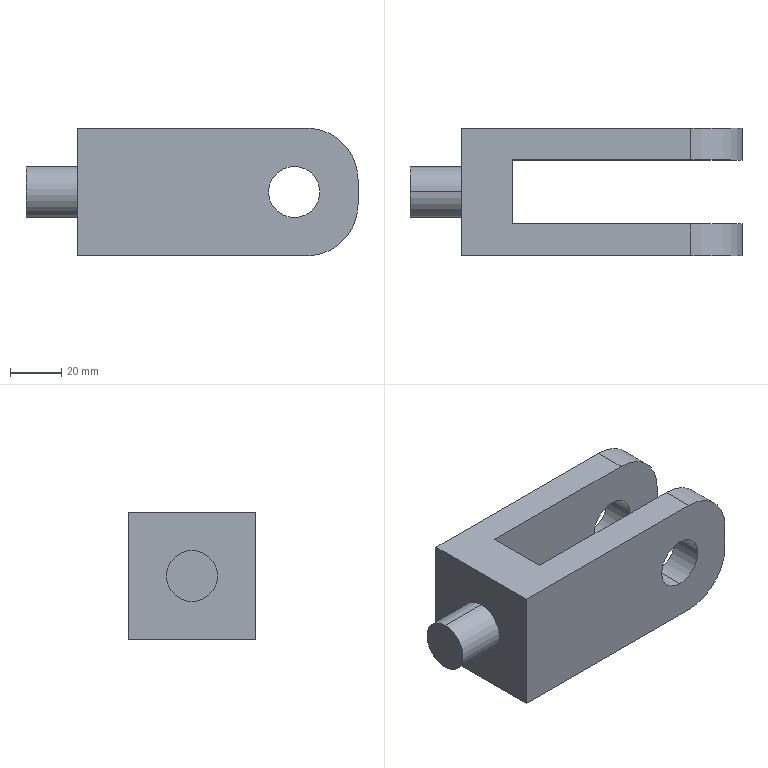Part | SolidWorks | 1 solid | 21 faces | box 130 x 50 x 50 mm | volume 156637 mm3 | plane 11 | cylinder 10 | commonest cylinder face diameters 20 x6 40 x4
STEP:
#1=CARTESIAN_POINT('',(-75.,25.,10.));
#2=VERTEX_POINT('',#1);
#3=CARTESIAN_POINT('',(-75.,25.,-10.));
#4=VERTEX_POINT('',#3);
#5=CARTESIAN_POINT('',(-75.,25.,0.));
#6=DIRECTION('',(-1.,0.,0.));
#7=DIRECTION('',(0.,0.,1.));
#8=AXIS2_PLACEMENT_3D('',#5,#6,#7);
#9=CIRCLE('',#8,10.);
#10=EDGE_CURVE('',#2,#4,#9,.T.);
#11=ORIENTED_EDGE('',*,*,#10,.F.);
#12=CARTESIAN_POINT('',(-55.,25.,10.));
#13=VERTEX_POINT('',#12);
#14=CARTESIAN_POINT('',(-75.,25.,10.));
#15=DIRECTION('',(1.,0.,0.));
#16=VECTOR('',#15,1000.);
#17=LINE('',#14,#16);
#18=EDGE_CURVE('',#2,#13,#17,.T.);
#19=ORIENTED_EDGE('',*,*,#18,.T.);
#20=CARTESIAN_POINT('',(-55.,25.,-10.));
#21=VERTEX_POINT('',#20);
#22=CARTESIAN_POINT('',(-55.,25.,0.));
#23=DIRECTION('',(-1.,0.,0.));
#24=DIRECTION('',(0.,0.,1.));
#25=AXIS2_PLACEMENT_3D('',#22,#23,#24);
#26=CIRCLE('',#25,10.);
#27=EDGE_CURVE('',#13,#21,#26,.T.);
#28=ORIENTED_EDGE('',*,*,#27,.T.);
#29=CARTESIAN_POINT('',(-75.,25.,-10.));
#30=DIRECTION('',(1.,0.,0.));
#31=VECTOR('',#30,1000.);
#32=LINE('',#29,#31);
#33=EDGE_CURVE('',#4,#21,#32,.T.);
#34=ORIENTED_EDGE('',*,*,#33,.F.);
#35=EDGE_LOOP('',(#11,#19,#28,#34));
#36=FACE_OUTER_BOUND('',#35,.T.);
#37=CARTESIAN_POINT('',(-75.,25.,0.));
#38=DIRECTION('',(1.,0.,0.));
#39=DIRECTION('',(0.,0.,-1.));
#40=AXIS2_PLACEMENT_3D('',#37,#38,#39);
#41=CYLINDRICAL_SURFACE('',#40,10.);
#42=ADVANCED_FACE('',(#36),#41,.T.);
#43=CARTESIAN_POINT('',(30.,12.5,10.));
#44=VERTEX_POINT('',#43);
#45=CARTESIAN_POINT('',(30.,12.5,-10.));
#46=VERTEX_POINT('',#45);
#47=CARTESIAN_POINT('',(30.,12.5,0.));
#48=DIRECTION('',(0.,-1.,0.));
#49=DIRECTION('',(0.,0.,-1.));
#50=AXIS2_PLACEMENT_3D('',#47,#48,#49);
#51=CIRCLE('',#50,10.);
#52=EDGE_CURVE('',#44,#46,#51,.T.);
#53=ORIENTED_EDGE('',*,*,#52,.F.);
#54=CARTESIAN_POINT('',(30.,0.,10.));
#55=VERTEX_POINT('',#54);
#56=CARTESIAN_POINT('',(30.,90.,10.));
#57=DIRECTION('',(0.,-1.,0.));
#58=VECTOR('',#57,1000.);
#59=LINE('',#56,#58);
#60=EDGE_CURVE('',#44,#55,#59,.T.);
#61=ORIENTED_EDGE('',*,*,#60,.T.);
#62=CARTESIAN_POINT('',(30.,0.,-10.));
#63=VERTEX_POINT('',#62);
#64=CARTESIAN_POINT('',(30.,0.,0.));
#65=DIRECTION('',(0.,-1.,0.));
#66=DIRECTION('',(0.,0.,-1.));
#67=AXIS2_PLACEMENT_3D('',#64,#65,#66);
#68=CIRCLE('',#67,10.);
#69=EDGE_CURVE('',#55,#63,#68,.T.);
#70=ORIENTED_EDGE('',*,*,#69,.T.);
#71=CARTESIAN_POINT('',(30.,90.,-10.));
#72=DIRECTION('',(0.,-1.,0.));
#73=VECTOR('',#72,1000.);
#74=LINE('',#71,#73);
#75=EDGE_CURVE('',#46,#63,#74,.T.);
#76=ORIENTED_EDGE('',*,*,#75,.F.);
#77=EDGE_LOOP('',(#53,#61,#70,#76));
#78=FACE_OUTER_BOUND('',#77,.T.);
#79=CARTESIAN_POINT('',(30.,90.,0.));
#80=DIRECTION('',(0.,-1.,0.));
#81=DIRECTION('',(0.,0.,-1.));
#82=AXIS2_PLACEMENT_3D('',#79,#80,#81);
#83=CYLINDRICAL_SURFACE('',#82,10.);
#84=ADVANCED_FACE('',(#78),#83,.F.);
#85=CARTESIAN_POINT('',(30.,50.,-10.));
#86=VERTEX_POINT('',#85);
#87=CARTESIAN_POINT('',(30.,50.,10.));
#88=VERTEX_POINT('',#87);
#89=CARTESIAN_POINT('',(30.,50.,0.));
#90=DIRECTION('',(0.,1.,0.));
#91=DIRECTION('',(0.,0.,1.));
#92=AXIS2_PLACEMENT_3D('',#89,#90,#91);
#93=CIRCLE('',#92,10.);
#94=EDGE_CURVE('',#86,#88,#93,.T.);
#95=ORIENTED_EDGE('',*,*,#94,.T.);
#96=CARTESIAN_POINT('',(30.,37.5,10.));
#97=VERTEX_POINT('',#96);
#98=CARTESIAN_POINT('',(30.,90.,10.));
#99=DIRECTION('',(0.,-1.,0.));
#100=VECTOR('',#99,1000.);
#101=LINE('',#98,#100);
#102=EDGE_CURVE('',#88,#97,#101,.T.);
#103=ORIENTED_EDGE('',*,*,#102,.T.);
#104=CARTESIAN_POINT('',(30.,37.5,-10.));
#105=VERTEX_POINT('',#104);
#106=CARTESIAN_POINT('',(30.,37.5,0.));
#107=DIRECTION('',(0.,1.,0.));
#108=DIRECTION('',(0.,0.,1.));
#109=AXIS2_PLACEMENT_3D('',#106,#107,#108);
#110=CIRCLE('',#109,10.);
#111=EDGE_CURVE('',#105,#97,#110,.T.);
#112=ORIENTED_EDGE('',*,*,#111,.F.);
#113=CARTESIAN_POINT('',(30.,90.,-10.));
#114=DIRECTION('',(0.,-1.,0.));
#115=VECTOR('',#114,1000.);
#116=LINE('',#113,#115);
#117=EDGE_CURVE('',#86,#105,#116,.T.);
#118=ORIENTED_EDGE('',*,*,#117,.F.);
#119=EDGE_LOOP('',(#95,#103,#112,#118));
#120=FACE_OUTER_BOUND('',#119,.T.);
#121=CARTESIAN_POINT('',(30.,90.,0.));
#122=DIRECTION('',(0.,-1.,0.));
#123=DIRECTION('',(0.,0.,-1.));
#124=AXIS2_PLACEMENT_3D('',#121,#122,#123);
#125=CYLINDRICAL_SURFACE('',#124,10.);
#126=ADVANCED_FACE('',(#120),#125,.F.);
#127=CARTESIAN_POINT('',(55.,0.,5.));
#128=VERTEX_POINT('',#127);
#129=CARTESIAN_POINT('',(55.,0.,-5.));
#130=VERTEX_POINT('',#129);
#131=CARTESIAN_POINT('',(55.,0.,-25.));
#132=DIRECTION('',(0.,0.,-1.));
#133=VECTOR('',#132,1000.);
#134=LINE('',#131,#133);
#135=EDGE_CURVE('',#128,#130,#134,.T.);
#136=ORIENTED_EDGE('',*,*,#135,.T.);
#137=CARTESIAN_POINT('',(55.,12.5,-5.));
#138=VERTEX_POINT('',#137);
#139=CARTESIAN_POINT('',(55.,50.,-5.));
#140=DIRECTION('',(0.,1.,0.));
#141=VECTOR('',#140,1000.);
#142=LINE('',#139,#141);
#143=EDGE_CURVE('',#130,#138,#142,.T.);
#144=ORIENTED_EDGE('',*,*,#143,.T.);
#145=CARTESIAN_POINT('',(55.,12.5,5.));
#146=VERTEX_POINT('',#145);
#147=CARTESIAN_POINT('',(55.,12.5,25.));
#148=DIRECTION('',(0.,0.,-1.));
#149=VECTOR('',#148,1000.);
#150=LINE('',#147,#149);
#151=EDGE_CURVE('',#146,#138,#150,.T.);
#152=ORIENTED_EDGE('',*,*,#151,.F.);
#153=CARTESIAN_POINT('',(55.,50.,5.));
#154=DIRECTION('',(0.,-1.,0.));
#155=VECTOR('',#154,1000.);
#156=LINE('',#153,#155);
#157=EDGE_CURVE('',#146,#128,#156,.T.);
#158=ORIENTED_EDGE('',*,*,#157,.T.);
#159=EDGE_LOOP('',(#136,#144,#152,#158));
#160=FACE_OUTER_BOUND('',#159,.T.);
#161=CARTESIAN_POINT('',(55.,50.,-25.));
#162=DIRECTION('',(-1.,0.,0.));
#163=DIRECTION('',(0.,0.,1.));
#164=AXIS2_PLACEMENT_3D('',#161,#162,#163);
#165=PLANE('',#164);
#166=ADVANCED_FACE('',(#160),#165,.F.);
#167=CARTESIAN_POINT('',(55.,37.5,-5.));
#168=VERTEX_POINT('',#167);
#169=CARTESIAN_POINT('',(55.,37.5,5.));
#170=VERTEX_POINT('',#169);
#171=CARTESIAN_POINT('',(55.,37.5,25.));
#172=DIRECTION('',(0.,0.,1.));
#173=VECTOR('',#172,1000.);
#174=LINE('',#171,#173);
#175=EDGE_CURVE('',#168,#170,#174,.T.);
#176=ORIENTED_EDGE('',*,*,#175,.F.);
#177=CARTESIAN_POINT('',(55.,50.,-5.));
#178=VERTEX_POINT('',#177);
#179=CARTESIAN_POINT('',(55.,50.,-5.));
#180=DIRECTION('',(0.,1.,0.));
#181=VECTOR('',#180,1000.);
#182=LINE('',#179,#181);
#183=EDGE_CURVE('',#168,#178,#182,.T.);
#184=ORIENTED_EDGE('',*,*,#183,.T.);
#185=CARTESIAN_POINT('',(55.,50.,5.));
#186=VERTEX_POINT('',#185);
#187=CARTESIAN_POINT('',(55.,50.,-25.));
#188=DIRECTION('',(0.,0.,-1.));
#189=VECTOR('',#188,1000.);
#190=LINE('',#187,#189);
#191=EDGE_CURVE('',#186,#178,#190,.T.);
#192=ORIENTED_EDGE('',*,*,#191,.F.);
#193=CARTESIAN_POINT('',(55.,50.,5.));
#194=DIRECTION('',(0.,-1.,0.));
#195=VECTOR('',#194,1000.);
#196=LINE('',#193,#195);
#197=EDGE_CURVE('',#186,#170,#196,.T.);
#198=ORIENTED_EDGE('',*,*,#197,.T.);
#199=EDGE_LOOP('',(#176,#184,#192,#198));
#200=FACE_OUTER_BOUND('',#199,.T.);
#201=CARTESIAN_POINT('',(55.,50.,-25.));
#202=DIRECTION('',(-1.,0.,0.));
#203=DIRECTION('',(0.,0.,1.));
#204=AXIS2_PLACEMENT_3D('',#201,#202,#203);
#205=PLANE('',#204);
#206=ADVANCED_FACE('',(#200),#205,.F.);
#207=CARTESIAN_POINT('',(-35.,12.5,-25.));
#208=VERTEX_POINT('',#207);
#209=CARTESIAN_POINT('',(35.,12.5,-25.));
#210=VERTEX_POINT('',#209);
#211=CARTESIAN_POINT('',(-35.,12.5,-25.));
#212=DIRECTION('',(1.,0.,0.));
#213=VECTOR('',#212,1000.);
#214=LINE('',#211,#213);
#215=EDGE_CURVE('',#208,#210,#214,.T.);
#216=ORIENTED_EDGE('',*,*,#215,.T.);
#217=CARTESIAN_POINT('',(35.,0.,-25.));
#218=VERTEX_POINT('',#217);
#219=CARTESIAN_POINT('',(35.,50.,-25.));
#220=DIRECTION('',(0.,-1.,0.));
#221=VECTOR('',#220,1000.);
#222=LINE('',#219,#221);
#223=EDGE_CURVE('',#210,#218,#222,.T.);
#224=ORIENTED_EDGE('',*,*,#223,.T.);
#225=CARTESIAN_POINT('',(-55.,0.,-25.));
#226=VERTEX_POINT('',#225);
#227=CARTESIAN_POINT('',(-55.,0.,-25.));
#228=DIRECTION('',(-1.,0.,0.));
#229=VECTOR('',#228,1000.);
#230=LINE('',#227,#229);
#231=EDGE_CURVE('',#218,#226,#230,.T.);
#232=ORIENTED_EDGE('',*,*,#231,.T.);
#233=CARTESIAN_POINT('',(-55.,50.,-25.));
#234=VERTEX_POINT('',#233);
#235=CARTESIAN_POINT('',(-55.,50.,-25.));
#236=DIRECTION('',(0.,-1.,0.));
#237=VECTOR('',#236,1000.);
#238=LINE('',#235,#237);
#239=EDGE_CURVE('',#234,#226,#238,.T.);
#240=ORIENTED_EDGE('',*,*,#239,.F.);
#241=CARTESIAN_POINT('',(35.,50.,-25.));
#242=VERTEX_POINT('',#241);
#243=CARTESIAN_POINT('',(-55.,50.,-25.));
#244=DIRECTION('',(-1.,0.,0.));
#245=VECTOR('',#244,1000.);
#246=LINE('',#243,#245);
#247=EDGE_CURVE('',#242,#234,#246,.T.);
#248=ORIENTED_EDGE('',*,*,#247,.F.);
#249=CARTESIAN_POINT('',(35.,37.5,-25.));
#250=VERTEX_POINT('',#249);
#251=CARTESIAN_POINT('',(35.,50.,-25.));
#252=DIRECTION('',(0.,-1.,0.));
#253=VECTOR('',#252,1000.);
#254=LINE('',#251,#253);
#255=EDGE_CURVE('',#242,#250,#254,.T.);
#256=ORIENTED_EDGE('',*,*,#255,.T.);
#257=CARTESIAN_POINT('',(-35.,37.5,-25.));
#258=VERTEX_POINT('',#257);
#259=CARTESIAN_POINT('',(-35.,37.5,-25.));
#260=DIRECTION('',(1.,0.,0.));
#261=VECTOR('',#260,1000.);
#262=LINE('',#259,#261);
#263=EDGE_CURVE('',#258,#250,#262,.T.);
#264=ORIENTED_EDGE('',*,*,#263,.F.);
#265=CARTESIAN_POINT('',(-35.,12.5,-25.));
#266=DIRECTION('',(0.,1.,0.));
#267=VECTOR('',#266,1000.);
#268=LINE('',#265,#267);
#269=EDGE_CURVE('',#208,#258,#268,.T.);
#270=ORIENTED_EDGE('',*,*,#269,.F.);
#271=EDGE_LOOP('',(#216,#224,#232,#240,#248,#256,#264,#270));
#272=FACE_OUTER_BOUND('',#271,.T.);
#273=CARTESIAN_POINT('',(-55.,50.,-25.));
#274=DIRECTION('',(0.,0.,1.));
#275=DIRECTION('',(1.,0.,0.));
#276=AXIS2_PLACEMENT_3D('',#273,#274,#275);
#277=PLANE('',#276);
#278=ADVANCED_FACE('',(#272),#277,.F.);
#279=CARTESIAN_POINT('',(-55.,25.,0.));
#280=DIRECTION('',(-1.,0.,0.));
#281=DIRECTION('',(0.,0.,1.));
#282=AXIS2_PLACEMENT_3D('',#279,#280,#281);
#283=CIRCLE('',#282,10.);
#284=EDGE_CURVE('',#21,#13,#283,.T.);
#285=ORIENTED_EDGE('',*,*,#284,.F.);
#286=ORIENTED_EDGE('',*,*,#27,.F.);
#287=EDGE_LOOP('',(#285,#286));
#288=FACE_BOUND('',#287,.T.);
#289=CARTESIAN_POINT('',(-55.,0.,25.));
#290=VERTEX_POINT('',#289);
#291=CARTESIAN_POINT('',(-55.,0.,-25.));
#292=DIRECTION('',(0.,0.,1.));
#293=VECTOR('',#292,1000.);
#294=LINE('',#291,#293);
#295=EDGE_CURVE('',#226,#290,#294,.T.);
#296=ORIENTED_EDGE('',*,*,#295,.T.);
#297=CARTESIAN_POINT('',(-55.,50.,25.));
#298=VERTEX_POINT('',#297);
#299=CARTESIAN_POINT('',(-55.,50.,25.));
#300=DIRECTION('',(0.,-1.,0.));
#301=VECTOR('',#300,1000.);
#302=LINE('',#299,#301);
#303=EDGE_CURVE('',#298,#290,#302,.T.);
#304=ORIENTED_EDGE('',*,*,#303,.F.);
#305=CARTESIAN_POINT('',(-55.,50.,-25.));
#306=DIRECTION('',(0.,0.,1.));
#307=VECTOR('',#306,1000.);
#308=LINE('',#305,#307);
#309=EDGE_CURVE('',#234,#298,#308,.T.);
#310=ORIENTED_EDGE('',*,*,#309,.F.);
#311=ORIENTED_EDGE('',*,*,#239,.T.);
#312=EDGE_LOOP('',(#296,#304,#310,#311));
#313=FACE_OUTER_BOUND('',#312,.T.);
#314=CARTESIAN_POINT('',(-55.,50.,-25.));
#315=DIRECTION('',(1.,0.,0.));
#316=DIRECTION('',(0.,0.,-1.));
#317=AXIS2_PLACEMENT_3D('',#314,#315,#316);
#318=PLANE('',#317);
#319=ADVANCED_FACE('',(#288,#313),#318,.F.);
#320=CARTESIAN_POINT('',(-35.,37.5,25.));
#321=VERTEX_POINT('',#320);
#322=CARTESIAN_POINT('',(35.,37.5,25.));
#323=VERTEX_POINT('',#322);
#324=CARTESIAN_POINT('',(-35.,37.5,25.));
#325=DIRECTION('',(1.,0.,0.));
#326=VECTOR('',#325,1000.);
#327=LINE('',#324,#326);
#328=EDGE_CURVE('',#321,#323,#327,.T.);
#329=ORIENTED_EDGE('',*,*,#328,.T.);
#330=CARTESIAN_POINT('',(35.,50.,25.));
#331=VERTEX_POINT('',#330);
#332=CARTESIAN_POINT('',(35.,50.,25.));
#333=DIRECTION('',(0.,1.,0.));
#334=VECTOR('',#333,1000.);
#335=LINE('',#332,#334);
#336=EDGE_CURVE('',#323,#331,#335,.T.);
#337=ORIENTED_EDGE('',*,*,#336,.T.);
#338=CARTESIAN_POINT('',(-55.,50.,25.));
#339=DIRECTION('',(1.,0.,0.));
#340=VECTOR('',#339,1000.);
#341=LINE('',#338,#340);
#342=EDGE_CURVE('',#298,#331,#341,.T.);
#343=ORIENTED_EDGE('',*,*,#342,.F.);
#344=ORIENTED_EDGE('',*,*,#303,.T.);
#345=CARTESIAN_POINT('',(35.,0.,25.));
#346=VERTEX_POINT('',#345);
#347=CARTESIAN_POINT('',(-55.,0.,25.));
#348=DIRECTION('',(1.,0.,0.));
#349=VECTOR('',#348,1000.);
#350=LINE('',#347,#349);
#351=EDGE_CURVE('',#290,#346,#350,.T.);
#352=ORIENTED_EDGE('',*,*,#351,.T.);
#353=CARTESIAN_POINT('',(35.,12.5,25.));
#354=VERTEX_POINT('',#353);
#355=CARTESIAN_POINT('',(35.,50.,25.));
#356=DIRECTION('',(0.,1.,0.));
#357=VECTOR('',#356,1000.);
#358=LINE('',#355,#357);
#359=EDGE_CURVE('',#346,#354,#358,.T.);
#360=ORIENTED_EDGE('',*,*,#359,.T.);
#361=CARTESIAN_POINT('',(-35.,12.5,25.));
#362=VERTEX_POINT('',#361);
#363=CARTESIAN_POINT('',(-35.,12.5,25.));
#364=DIRECTION('',(1.,0.,0.));
#365=VECTOR('',#364,1000.);
#366=LINE('',#363,#365);
#367=EDGE_CURVE('',#362,#354,#366,.T.);
#368=ORIENTED_EDGE('',*,*,#367,.F.);
#369=CARTESIAN_POINT('',(-35.,12.5,25.));
#370=DIRECTION('',(0.,-1.,0.));
#371=VECTOR('',#370,1000.);
#372=LINE('',#369,#371);
#373=EDGE_CURVE('',#321,#362,#372,.T.);
#374=ORIENTED_EDGE('',*,*,#373,.F.);
#375=EDGE_LOOP('',(#329,#337,#343,#344,#352,#360,#368,#374));
#376=FACE_OUTER_BOUND('',#375,.T.);
#377=CARTESIAN_POINT('',(-55.,50.,25.));
#378=DIRECTION('',(0.,0.,-1.));
#379=DIRECTION('',(-1.,0.,0.));
#380=AXIS2_PLACEMENT_3D('',#377,#378,#379);
#381=PLANE('',#380);
#382=ADVANCED_FACE('',(#376),#381,.F.);
#383=ORIENTED_EDGE('',*,*,#94,.F.);
#384=CARTESIAN_POINT('',(30.,50.,0.));
#385=DIRECTION('',(0.,1.,0.));
#386=DIRECTION('',(0.,0.,1.));
#387=AXIS2_PLACEMENT_3D('',#384,#385,#386);
#388=CIRCLE('',#387,10.);
#389=EDGE_CURVE('',#88,#86,#388,.T.);
#390=ORIENTED_EDGE('',*,*,#389,.F.);
#391=EDGE_LOOP('',(#383,#390));
#392=FACE_BOUND('',#391,.T.);
#393=ORIENTED_EDGE('',*,*,#191,.T.);
#394=CARTESIAN_POINT('',(35.,50.,-5.));
#395=DIRECTION('',(0.,1.,0.));
#396=DIRECTION('',(0.,0.,1.));
#397=AXIS2_PLACEMENT_3D('',#394,#395,#396);
#398=CIRCLE('',#397,20.);
#399=EDGE_CURVE('',#178,#242,#398,.T.);
#400=ORIENTED_EDGE('',*,*,#399,.T.);
#401=ORIENTED_EDGE('',*,*,#247,.T.);
#402=ORIENTED_EDGE('',*,*,#309,.T.);
#403=ORIENTED_EDGE('',*,*,#342,.T.);
#404=CARTESIAN_POINT('',(35.,50.,5.));
#405=DIRECTION('',(0.,1.,0.));
#406=DIRECTION('',(0.,0.,1.));
#407=AXIS2_PLACEMENT_3D('',#404,#405,#406);
#408=CIRCLE('',#407,20.);
#409=EDGE_CURVE('',#331,#186,#408,.T.);
#410=ORIENTED_EDGE('',*,*,#409,.T.);
#411=EDGE_LOOP('',(#393,#400,#401,#402,#403,#410));
#412=FACE_OUTER_BOUND('',#411,.T.);
#413=CARTESIAN_POINT('',(0.,50.,0.));
#414=DIRECTION('',(0.,1.,0.));
#415=DIRECTION('',(0.,0.,1.));
#416=AXIS2_PLACEMENT_3D('',#413,#414,#415);
#417=PLANE('',#416);
#418=ADVANCED_FACE('',(#392,#412),#417,.T.);
#419=CARTESIAN_POINT('',(30.,0.,0.));
#420=DIRECTION('',(0.,-1.,0.));
#421=DIRECTION('',(0.,0.,-1.));
#422=AXIS2_PLACEMENT_3D('',#419,#420,#421);
#423=CIRCLE('',#422,10.);
#424=EDGE_CURVE('',#63,#55,#423,.T.);
#425=ORIENTED_EDGE('',*,*,#424,.F.);
#426=ORIENTED_EDGE('',*,*,#69,.F.);
#427=EDGE_LOOP('',(#425,#426));
#428=FACE_BOUND('',#427,.T.);
#429=ORIENTED_EDGE('',*,*,#231,.F.);
#430=CARTESIAN_POINT('',(35.,0.,-5.));
#431=DIRECTION('',(0.,-1.,0.));
#432=DIRECTION('',(0.,0.,1.));
#433=AXIS2_PLACEMENT_3D('',#430,#431,#432);
#434=CIRCLE('',#433,20.);
#435=EDGE_CURVE('',#218,#130,#434,.T.);
#436=ORIENTED_EDGE('',*,*,#435,.T.);
#437=ORIENTED_EDGE('',*,*,#135,.F.);
#438=CARTESIAN_POINT('',(35.,0.,5.));
#439=DIRECTION('',(0.,-1.,0.));
#440=DIRECTION('',(0.,0.,1.));
#441=AXIS2_PLACEMENT_3D('',#438,#439,#440);
#442=CIRCLE('',#441,20.);
#443=EDGE_CURVE('',#128,#346,#442,.T.);
#444=ORIENTED_EDGE('',*,*,#443,.T.);
#445=ORIENTED_EDGE('',*,*,#351,.F.);
#446=ORIENTED_EDGE('',*,*,#295,.F.);
#447=EDGE_LOOP('',(#429,#436,#437,#444,#445,#446));
#448=FACE_OUTER_BOUND('',#447,.T.);
#449=CARTESIAN_POINT('',(0.,0.,0.));
#450=DIRECTION('',(0.,1.,0.));
#451=DIRECTION('',(0.,0.,1.));
#452=AXIS2_PLACEMENT_3D('',#449,#450,#451);
#453=PLANE('',#452);
#454=ADVANCED_FACE('',(#428,#448),#453,.F.);
#455=CARTESIAN_POINT('',(30.,12.5,0.));
#456=DIRECTION('',(0.,-1.,0.));
#457=DIRECTION('',(0.,0.,-1.));
#458=AXIS2_PLACEMENT_3D('',#455,#456,#457);
#459=CIRCLE('',#458,10.);
#460=EDGE_CURVE('',#46,#44,#459,.T.);
#461=ORIENTED_EDGE('',*,*,#460,.T.);
#462=ORIENTED_EDGE('',*,*,#52,.T.);
#463=EDGE_LOOP('',(#461,#462));
#464=FACE_BOUND('',#463,.T.);
#465=ORIENTED_EDGE('',*,*,#151,.T.);
#466=CARTESIAN_POINT('',(35.,12.5,-5.));
#467=DIRECTION('',(0.,1.,0.));
#468=DIRECTION('',(0.,0.,-1.));
#469=AXIS2_PLACEMENT_3D('',#466,#467,#468);
#470=CIRCLE('',#469,20.);
#471=EDGE_CURVE('',#138,#210,#470,.T.);
#472=ORIENTED_EDGE('',*,*,#471,.T.);
#473=ORIENTED_EDGE('',*,*,#215,.F.);
#474=CARTESIAN_POINT('',(-35.,12.5,25.));
#475=DIRECTION('',(0.,0.,-1.));
#476=VECTOR('',#475,1000.);
#477=LINE('',#474,#476);
#478=EDGE_CURVE('',#362,#208,#477,.T.);
#479=ORIENTED_EDGE('',*,*,#478,.F.);
#480=ORIENTED_EDGE('',*,*,#367,.T.);
#481=CARTESIAN_POINT('',(35.,12.5,5.));
#482=DIRECTION('',(0.,1.,0.));
#483=DIRECTION('',(0.,0.,-1.));
#484=AXIS2_PLACEMENT_3D('',#481,#482,#483);
#485=CIRCLE('',#484,20.);
#486=EDGE_CURVE('',#354,#146,#485,.T.);
#487=ORIENTED_EDGE('',*,*,#486,.T.);
#488=EDGE_LOOP('',(#465,#472,#473,#479,#480,#487));
#489=FACE_OUTER_BOUND('',#488,.T.);
#490=CARTESIAN_POINT('',(-35.,12.5,25.));
#491=DIRECTION('',(0.,-1.,0.));
#492=DIRECTION('',(0.,0.,-1.));
#493=AXIS2_PLACEMENT_3D('',#490,#491,#492);
#494=PLANE('',#493);
#495=ADVANCED_FACE('',(#464,#489),#494,.F.);
#496=ORIENTED_EDGE('',*,*,#111,.T.);
#497=CARTESIAN_POINT('',(30.,37.5,0.));
#498=DIRECTION('',(0.,1.,0.));
#499=DIRECTION('',(0.,0.,1.));
#500=AXIS2_PLACEMENT_3D('',#497,#498,#499);
#501=CIRCLE('',#500,10.);
#502=EDGE_CURVE('',#97,#105,#501,.T.);
#503=ORIENTED_EDGE('',*,*,#502,.T.);
#504=EDGE_LOOP('',(#496,#503));
#505=FACE_BOUND('',#504,.T.);
#506=ORIENTED_EDGE('',*,*,#263,.T.);
#507=CARTESIAN_POINT('',(35.,37.5,-5.));
#508=DIRECTION('',(0.,-1.,0.));
#509=DIRECTION('',(0.,0.,1.));
#510=AXIS2_PLACEMENT_3D('',#507,#508,#509);
#511=CIRCLE('',#510,20.);
#512=EDGE_CURVE('',#250,#168,#511,.T.);
#513=ORIENTED_EDGE('',*,*,#512,.T.);
#514=ORIENTED_EDGE('',*,*,#175,.T.);
#515=CARTESIAN_POINT('',(35.,37.5,5.));
#516=DIRECTION('',(0.,-1.,0.));
#517=DIRECTION('',(0.,0.,1.));
#518=AXIS2_PLACEMENT_3D('',#515,#516,#517);
#519=CIRCLE('',#518,20.);
#520=EDGE_CURVE('',#170,#323,#519,.T.);
#521=ORIENTED_EDGE('',*,*,#520,.T.);
#522=ORIENTED_EDGE('',*,*,#328,.F.);
#523=CARTESIAN_POINT('',(-35.,37.5,25.));
#524=DIRECTION('',(0.,0.,1.));
#525=VECTOR('',#524,1000.);
#526=LINE('',#523,#525);
#527=EDGE_CURVE('',#258,#321,#526,.T.);
#528=ORIENTED_EDGE('',*,*,#527,.F.);
#529=EDGE_LOOP('',(#506,#513,#514,#521,#522,#528));
#530=FACE_OUTER_BOUND('',#529,.T.);
#531=CARTESIAN_POINT('',(-35.,37.5,25.));
#532=DIRECTION('',(0.,1.,0.));
#533=DIRECTION('',(0.,0.,1.));
#534=AXIS2_PLACEMENT_3D('',#531,#532,#533);
#535=PLANE('',#534);
#536=ADVANCED_FACE('',(#505,#530),#535,.F.);
#537=ORIENTED_EDGE('',*,*,#269,.T.);
#538=ORIENTED_EDGE('',*,*,#527,.T.);
#539=ORIENTED_EDGE('',*,*,#373,.T.);
#540=ORIENTED_EDGE('',*,*,#478,.T.);
#541=EDGE_LOOP('',(#537,#538,#539,#540));
#542=FACE_OUTER_BOUND('',#541,.T.);
#543=CARTESIAN_POINT('',(-35.,0.,0.));
#544=DIRECTION('',(-1.,0.,0.));
#545=DIRECTION('',(0.,0.,1.));
#546=AXIS2_PLACEMENT_3D('',#543,#544,#545);
#547=PLANE('',#546);
#548=ADVANCED_FACE('',(#542),#547,.F.);
#549=ORIENTED_EDGE('',*,*,#471,.F.);
#550=ORIENTED_EDGE('',*,*,#143,.F.);
#551=ORIENTED_EDGE('',*,*,#435,.F.);
#552=ORIENTED_EDGE('',*,*,#223,.F.);
#553=EDGE_LOOP('',(#549,#550,#551,#552));
#554=FACE_OUTER_BOUND('',#553,.T.);
#555=CARTESIAN_POINT('',(35.,50.,-5.));
#556=DIRECTION('',(0.,-1.,0.));
#557=DIRECTION('',(0.,0.,-1.));
#558=AXIS2_PLACEMENT_3D('',#555,#556,#557);
#559=CYLINDRICAL_SURFACE('',#558,20.);
#560=ADVANCED_FACE('',(#554),#559,.T.);
#561=ORIENTED_EDGE('',*,*,#399,.F.);
#562=ORIENTED_EDGE('',*,*,#183,.F.);
#563=ORIENTED_EDGE('',*,*,#512,.F.);
#564=ORIENTED_EDGE('',*,*,#255,.F.);
#565=EDGE_LOOP('',(#561,#562,#563,#564));
#566=FACE_OUTER_BOUND('',#565,.T.);
#567=CARTESIAN_POINT('',(35.,50.,-5.));
#568=DIRECTION('',(0.,-1.,0.));
#569=DIRECTION('',(0.,0.,-1.));
#570=AXIS2_PLACEMENT_3D('',#567,#568,#569);
#571=CYLINDRICAL_SURFACE('',#570,20.);
#572=ADVANCED_FACE('',(#566),#571,.T.);
#573=ORIENTED_EDGE('',*,*,#409,.F.);
#574=ORIENTED_EDGE('',*,*,#336,.F.);
#575=ORIENTED_EDGE('',*,*,#520,.F.);
#576=ORIENTED_EDGE('',*,*,#197,.F.);
#577=EDGE_LOOP('',(#573,#574,#575,#576));
#578=FACE_OUTER_BOUND('',#577,.T.);
#579=CARTESIAN_POINT('',(35.,50.,5.));
#580=DIRECTION('',(0.,-1.,0.));
#581=DIRECTION('',(0.,0.,-1.));
#582=AXIS2_PLACEMENT_3D('',#579,#580,#581);
#583=CYLINDRICAL_SURFACE('',#582,20.);
#584=ADVANCED_FACE('',(#578),#583,.T.);
#585=ORIENTED_EDGE('',*,*,#486,.F.);
#586=ORIENTED_EDGE('',*,*,#359,.F.);
#587=ORIENTED_EDGE('',*,*,#443,.F.);
#588=ORIENTED_EDGE('',*,*,#157,.F.);
#589=EDGE_LOOP('',(#585,#586,#587,#588));
#590=FACE_OUTER_BOUND('',#589,.T.);
#591=CARTESIAN_POINT('',(35.,50.,5.));
#592=DIRECTION('',(0.,-1.,0.));
#593=DIRECTION('',(0.,0.,-1.));
#594=AXIS2_PLACEMENT_3D('',#591,#592,#593);
#595=CYLINDRICAL_SURFACE('',#594,20.);
#596=ADVANCED_FACE('',(#590),#595,.T.);
#597=ORIENTED_EDGE('',*,*,#102,.F.);
#598=ORIENTED_EDGE('',*,*,#389,.T.);
#599=ORIENTED_EDGE('',*,*,#117,.T.);
#600=ORIENTED_EDGE('',*,*,#502,.F.);
#601=EDGE_LOOP('',(#597,#598,#599,#600));
#602=FACE_OUTER_BOUND('',#601,.T.);
#603=CARTESIAN_POINT('',(30.,90.,0.));
#604=DIRECTION('',(0.,-1.,0.));
#605=DIRECTION('',(0.,0.,-1.));
#606=AXIS2_PLACEMENT_3D('',#603,#604,#605);
#607=CYLINDRICAL_SURFACE('',#606,10.);
#608=ADVANCED_FACE('',(#602),#607,.F.);
#609=ORIENTED_EDGE('',*,*,#60,.F.);
#610=ORIENTED_EDGE('',*,*,#460,.F.);
#611=ORIENTED_EDGE('',*,*,#75,.T.);
#612=ORIENTED_EDGE('',*,*,#424,.T.);
#613=EDGE_LOOP('',(#609,#610,#611,#612));
#614=FACE_OUTER_BOUND('',#613,.T.);
#615=CARTESIAN_POINT('',(30.,90.,0.));
#616=DIRECTION('',(0.,-1.,0.));
#617=DIRECTION('',(0.,0.,-1.));
#618=AXIS2_PLACEMENT_3D('',#615,#616,#617);
#619=CYLINDRICAL_SURFACE('',#618,10.);
#620=ADVANCED_FACE('',(#614),#619,.F.);
#621=ORIENTED_EDGE('',*,*,#18,.F.);
#622=CARTESIAN_POINT('',(-75.,25.,0.));
#623=DIRECTION('',(-1.,0.,0.));
#624=DIRECTION('',(0.,0.,1.));
#625=AXIS2_PLACEMENT_3D('',#622,#623,#624);
#626=CIRCLE('',#625,10.);
#627=EDGE_CURVE('',#4,#2,#626,.T.);
#628=ORIENTED_EDGE('',*,*,#627,.F.);
#629=ORIENTED_EDGE('',*,*,#33,.T.);
#630=ORIENTED_EDGE('',*,*,#284,.T.);
#631=EDGE_LOOP('',(#621,#628,#629,#630));
#632=FACE_OUTER_BOUND('',#631,.T.);
#633=CARTESIAN_POINT('',(-75.,25.,0.));
#634=DIRECTION('',(1.,0.,0.));
#635=DIRECTION('',(0.,0.,-1.));
#636=AXIS2_PLACEMENT_3D('',#633,#634,#635);
#637=CYLINDRICAL_SURFACE('',#636,10.);
#638=ADVANCED_FACE('',(#632),#637,.T.);
#639=ORIENTED_EDGE('',*,*,#627,.T.);
#640=ORIENTED_EDGE('',*,*,#10,.T.);
#641=EDGE_LOOP('',(#639,#640));
#642=FACE_OUTER_BOUND('',#641,.T.);
#643=CARTESIAN_POINT('',(-75.,25.,0.));
#644=DIRECTION('',(-1.,0.,0.));
#645=DIRECTION('',(0.,0.,1.));
#646=AXIS2_PLACEMENT_3D('',#643,#644,#645);
#647=PLANE('',#646);
#648=ADVANCED_FACE('',(#642),#647,.T.);
#649=CLOSED_SHELL('',(#42,#84,#126,#166,#206,#278,#319,#382,#418,#454,#495,#536,#548,#560,#572,#584,#596,#608,#620,#638,#648));
#650=MANIFOLD_SOLID_BREP('',#649);
#651=CARTESIAN_POINT('',(0.,0.,0.));
#652=DIRECTION('',(0.,0.,1.));
#653=DIRECTION('',(1.,0.,0.));
#654=AXIS2_PLACEMENT_3D('',#651,#652,#653);
#655=(LENGTH_UNIT()NAMED_UNIT(*)SI_UNIT(.MILLI.,.METRE.));
#656=UNCERTAINTY_MEASURE_WITH_UNIT(LENGTH_MEASURE(0.00001),#655,'','');
#657=(NAMED_UNIT(*)PLANE_ANGLE_UNIT()SI_UNIT($,.RADIAN.));
#658=(NAMED_UNIT(*)SI_UNIT($,.STERADIAN.)SOLID_ANGLE_UNIT());
#659=(GEOMETRIC_REPRESENTATION_CONTEXT(3)GLOBAL_UNCERTAINTY_ASSIGNED_CONTEXT((#656))GLOBAL_UNIT_ASSIGNED_CONTEXT((#655,#657,#658))REPRESENTATION_CONTEXT('',''));
#660=ADVANCED_BREP_SHAPE_REPRESENTATION('',(#650,#654),#659);